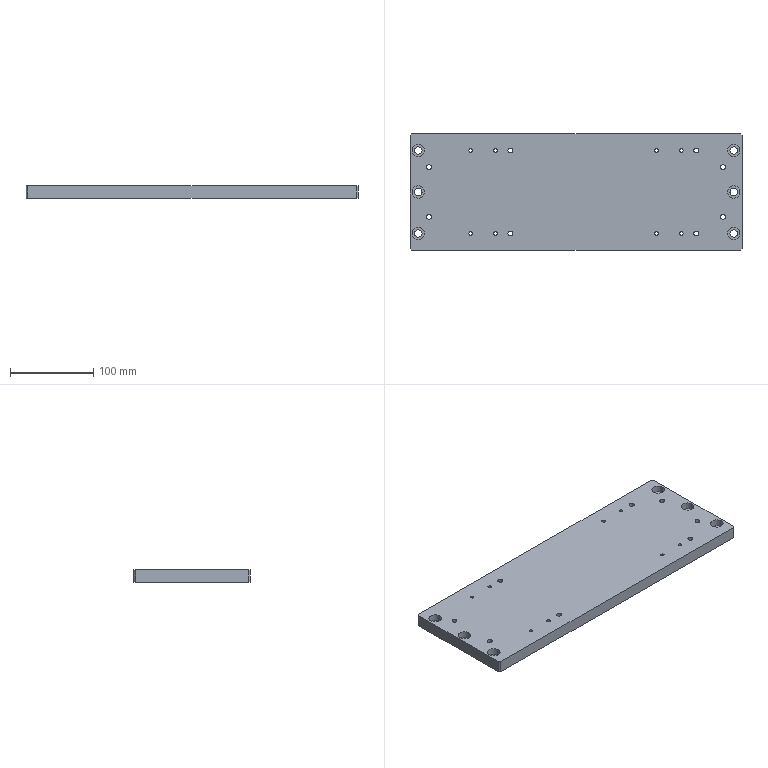CAM job | NX | 3-axis milling, drilling | part box 400 x 140 x 15 mm | stock box 400 x 140 x 15 mm
Tools:
number,name,description,diameter,corner_radius,flute_length,length,flutes
8,D8,平底铣刀-粗,8.0,0.0,30.0,75.0,2
9,D10,平底铣刀-粗,10.0,0.0,35.0,75.0,2
7,D6-J,平底铣刀-精,6.0,0.0,25.0,75.0,2
10,D10-J,平底铣刀-精,10.0,0.0,35.0,75.0,2
2,D6倒角刀,倒角刀,6.0,0.0,3.0,25.0,2
22,M5X0.8,丝锥,4.2,0.0,35.0,50.0,2
19,D6铰刀,Drilling Tool,6.0,0.0,75.0,100.0,6
1,C6定点钻,倒角刀,6.0,0.0,3.0,3.0,2
17,ZT9,钻头,9.0,0.0,35.0,50.0,2
14,ZT4.3,Drilling Tool,4.3,0.0,50.0,75.0,4
18,ZT5.9,Drilling Tool,5.9,0.0,35.0,50.0,2
Operations:
program,operation,operation_type,tool,method,geometry_group,spindle_rpm,surface_speed,feed_per_tooth,feed_cut,feed_plunge,cut_length_mm,path_length_mm,cut_time_min,machine_time_min
B,选线往复层切开粗-中_COPY_1,PlanarMilling,D10,分层开粗-切深K-步距G,W-B,3000.0,94.245,0.3333,2000.0,100.0,1333.019,2493.614,0.6665,0.7826
B,钻倒角_1,Operation,D6倒角刀,METHOD,W-B,2000.0,0.0,0.025,100.0,0.0,45.6,726.912,0.456,0.5241
B,平面去毛刺6X45L_COPY_1,SurfaceContour,D6倒角刀,爬面_倒角-切深0-步距G,W-B,3500.0,65.972,0.1429,1000.0,100.0,1457.772,3075.395,1.458,1.619
B,平面铣精光侧面-中-直线_COPY_1,PlanarMilling,D10-J,侧刃精光-切深K-步距G,W-B,3000.0,94.245,0.1333,800.0,100.0,67.314,1187.071,0.0841,0.1961
A,选线往复层切开粗-中_COPY,PlanarMilling,D10,分层开粗-切深K-步距G,W-A,3000.0,94.245,0.3333,2000.0,100.0,1333.019,2493.614,0.6665,0.7826
A,打点-深0.8,Operation,C6定点钻,NONE,W-A,3000.0,56.0,0.01,60.0,90.0,39.6,1010.761,0.66,0.7571
A,沉头孔-钻孔0段,Operation,ZT9,NONE,W-A,500.0,14.137,0.12,120.0,90.0,124.223,933.488,1.035,1.116
A,通孔-M5螺纹底孔,Operation,ZT4.3,NONE,W-A,1200.0,15.834,0.0333,80.0,90.0,176.0,973.079,2.2,2.28
A,通孔-精孔6.0预钻,Operation,ZT5.9,NONE,W-A,1000.0,18.221,0.04,80.0,90.0,168.0,1062.547,2.1,2.189
A,铣孔开粗D8_1,CylinderMilling,D8,NONE,W-A,4000.0,100.531,0.25,2000.0,100.0,4858.227,6136.827,2.429,2.557
A,铣孔精光D8_1,CylinderMilling,D6-J,精光步距切深关,W-A,4000.0,100.531,0.1,800.0,100.0,561.894,1840.494,0.7024,0.8302
A,铣倒角_1,PlanarMilling,D6倒角刀,METHOD,W-A,4000.0,75.398,0.025,200.0,100.0,144.163,1466.296,0.7208,0.853
A,平面去毛刺6X45L_COPY,SurfaceContour,D6倒角刀,爬面_倒角-切深0-步距G,W-A,3500.0,65.972,0.1429,1000.0,100.0,1800.081,4233.705,1.8,2.043
A,通孔-攻牙M5,Operation,M5X0.8,METHOD,W-A,500.0,6.597,0.0008,0.8,90.0,152.0,925.079,190.0,190.077
A,铰孔,Operation,D6铰刀,METHOD,W-A,500.0,9.425,0.0167,50.0,0.0,136.0,998.547,2.72,2.806
A,平面铣精光侧面-中-直线_COPY,PlanarMilling,D10-J,侧刃精光-切深K-步距G,W-A,3000.0,94.245,0.1333,800.0,100.0,67.314,1187.071,0.0841,0.1961